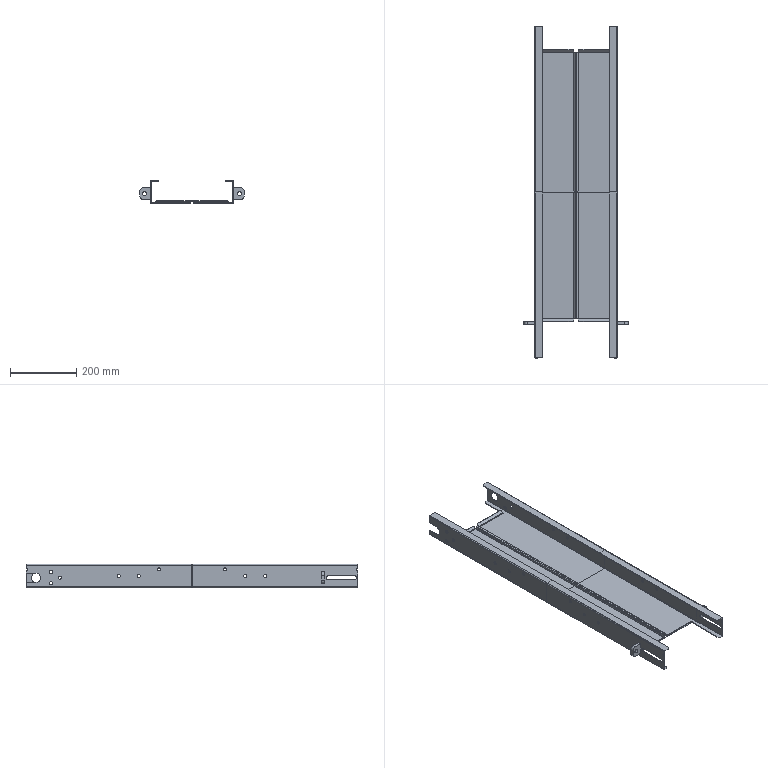Part | STEP file | MM-P41130-01_1 | 6 solids | 216 faces | box 314 x 1000 x 70 mm | volume 800616 mm3 | cylinder 111 | plane 105 | commonest cylinder face diameters 9 x28 10 x28 1.473 x20 5.473 x20 11 x4 12.5 x4